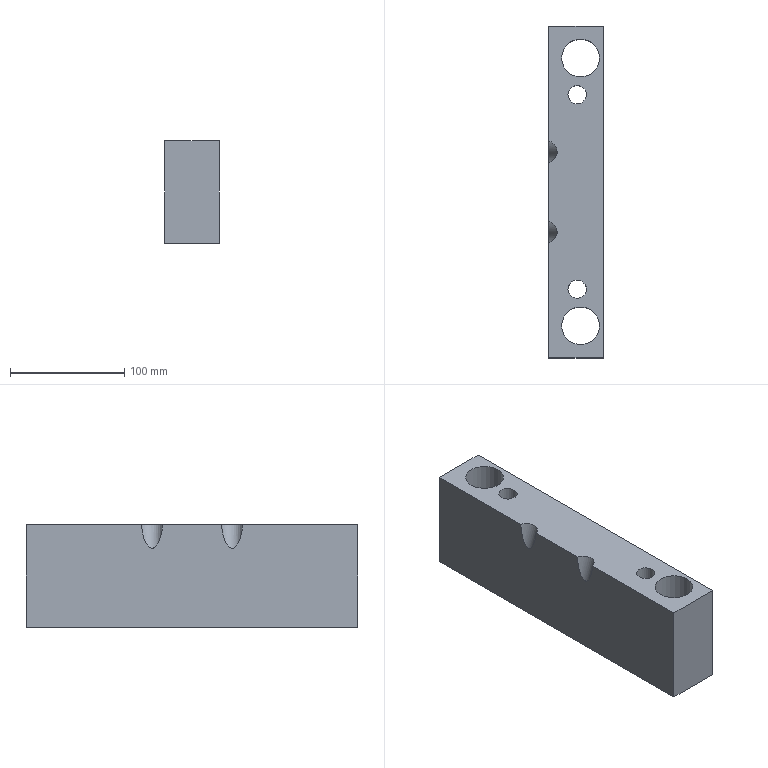Part | STEP file | CC01_id270_x_t | 1 solid | 18 faces | box 48 x 290 x 90 mm | volume 1057434 mm3 | plane 8 | cylinder 8 | cone 2 | commonest cylinder face diameters 10 x2 16 x2 20 x2 33 x2
STEP:
#1=CARTESIAN_POINT('',(-125.,44.563,-75.5));
#2=VERTEX_POINT('',#1);
#3=CARTESIAN_POINT('',(-125.,25.437,-75.5));
#4=VERTEX_POINT('',#3);
#5=CARTESIAN_POINT('',(-125.,35.,-66.95));
#6=DIRECTION('',(-1.,0.,0.));
#7=DIRECTION('',(0.,0.,1.));
#8=AXIS2_PLACEMENT_3D('',#5,#6,#7);
#9=ELLIPSE('',#8,29.238,10.);
#10=EDGE_CURVE('',#2,#4,#9,.T.);
#11=ORIENTED_EDGE('',*,*,#10,.F.);
#12=CARTESIAN_POINT('',(-125.,145.,-75.5));
#13=VERTEX_POINT('',#12);
#14=CARTESIAN_POINT('',(-125.,0.,-75.5));
#15=DIRECTION('',(0.,1.,0.));
#16=VECTOR('',#15,1.);
#17=LINE('',#14,#16);
#18=EDGE_CURVE('',#2,#13,#17,.T.);
#19=ORIENTED_EDGE('',*,*,#18,.T.);
#20=CARTESIAN_POINT('',(-125.,145.,-165.5));
#21=VERTEX_POINT('',#20);
#22=CARTESIAN_POINT('',(-125.,145.,-165.5));
#23=DIRECTION('',(0.,0.,1.));
#24=VECTOR('',#23,1.);
#25=LINE('',#22,#24);
#26=EDGE_CURVE('',#21,#13,#25,.T.);
#27=ORIENTED_EDGE('',*,*,#26,.F.);
#28=CARTESIAN_POINT('',(-125.,-145.,-165.5));
#29=VERTEX_POINT('',#28);
#30=CARTESIAN_POINT('',(-125.,0.,-165.5));
#31=DIRECTION('',(0.,-1.,0.));
#32=VECTOR('',#31,1.);
#33=LINE('',#30,#32);
#34=EDGE_CURVE('',#21,#29,#33,.T.);
#35=ORIENTED_EDGE('',*,*,#34,.T.);
#36=CARTESIAN_POINT('',(-125.,-145.,-75.5));
#37=VERTEX_POINT('',#36);
#38=CARTESIAN_POINT('',(-125.,-145.,-165.5));
#39=DIRECTION('',(0.,0.,1.));
#40=VECTOR('',#39,1.);
#41=LINE('',#38,#40);
#42=EDGE_CURVE('',#29,#37,#41,.T.);
#43=ORIENTED_EDGE('',*,*,#42,.T.);
#44=CARTESIAN_POINT('',(-125.,-44.563,-75.5));
#45=VERTEX_POINT('',#44);
#46=CARTESIAN_POINT('',(-125.,0.,-75.5));
#47=DIRECTION('',(0.,1.,0.));
#48=VECTOR('',#47,1.);
#49=LINE('',#46,#48);
#50=EDGE_CURVE('',#37,#45,#49,.T.);
#51=ORIENTED_EDGE('',*,*,#50,.T.);
#52=CARTESIAN_POINT('',(-125.,-25.437,-75.5));
#53=VERTEX_POINT('',#52);
#54=CARTESIAN_POINT('',(-125.,-35.,-66.95));
#55=DIRECTION('',(-1.,0.,0.));
#56=DIRECTION('',(0.,0.,1.));
#57=AXIS2_PLACEMENT_3D('',#54,#55,#56);
#58=ELLIPSE('',#57,29.238,10.);
#59=EDGE_CURVE('',#53,#45,#58,.T.);
#60=ORIENTED_EDGE('',*,*,#59,.F.);
#61=CARTESIAN_POINT('',(-125.,0.,-75.5));
#62=DIRECTION('',(0.,1.,0.));
#63=VECTOR('',#62,1.);
#64=LINE('',#61,#63);
#65=EDGE_CURVE('',#53,#4,#64,.T.);
#66=ORIENTED_EDGE('',*,*,#65,.T.);
#67=EDGE_LOOP('',(#11,#19,#27,#35,#43,#51,#60,#66));
#68=FACE_OUTER_BOUND('',#67,.T.);
#69=CARTESIAN_POINT('',(-125.,0.,-165.5));
#70=DIRECTION('',(-1.,0.,0.));
#71=DIRECTION('',(0.,0.,1.));
#72=AXIS2_PLACEMENT_3D('',#69,#70,#71);
#73=PLANE('',#72);
#74=ADVANCED_FACE('',(#68),#73,.T.);
#75=CARTESIAN_POINT('',(-113.5,-117.,-165.5));
#76=VERTEX_POINT('',#75);
#77=CARTESIAN_POINT('',(-97.,-117.,-165.5));
#78=DIRECTION('',(0.,0.,1.));
#79=DIRECTION('',(-1.,0.,0.));
#80=AXIS2_PLACEMENT_3D('',#77,#78,#79);
#81=CIRCLE('',#80,16.5);
#82=EDGE_CURVE('',#76,#76,#81,.T.);
#83=ORIENTED_EDGE('',*,*,#82,.T.);
#84=EDGE_LOOP('',(#83));
#85=FACE_BOUND('',#84,.T.);
#86=CARTESIAN_POINT('',(-95.,40.,-165.5));
#87=VERTEX_POINT('',#86);
#88=CARTESIAN_POINT('',(-100.,40.,-165.5));
#89=DIRECTION('',(0.,0.,1.));
#90=DIRECTION('',(1.,0.,0.));
#91=AXIS2_PLACEMENT_3D('',#88,#89,#90);
#92=CIRCLE('',#91,5.);
#93=EDGE_CURVE('',#87,#87,#92,.T.);
#94=ORIENTED_EDGE('',*,*,#93,.T.);
#95=EDGE_LOOP('',(#94));
#96=FACE_BOUND('',#95,.T.);
#97=CARTESIAN_POINT('',(-92.,85.,-165.5));
#98=VERTEX_POINT('',#97);
#99=CARTESIAN_POINT('',(-100.,85.,-165.5));
#100=DIRECTION('',(0.,0.,1.));
#101=DIRECTION('',(1.,0.,0.));
#102=AXIS2_PLACEMENT_3D('',#99,#100,#101);
#103=CIRCLE('',#102,8.);
#104=EDGE_CURVE('',#98,#98,#103,.T.);
#105=ORIENTED_EDGE('',*,*,#104,.T.);
#106=EDGE_LOOP('',(#105));
#107=FACE_BOUND('',#106,.T.);
#108=CARTESIAN_POINT('',(-77.,-145.,-165.5));
#109=VERTEX_POINT('',#108);
#110=CARTESIAN_POINT('',(-77.,145.,-165.5));
#111=VERTEX_POINT('',#110);
#112=CARTESIAN_POINT('',(-77.,0.,-165.5));
#113=DIRECTION('',(0.,1.,0.));
#114=VECTOR('',#113,1.);
#115=LINE('',#112,#114);
#116=EDGE_CURVE('',#109,#111,#115,.T.);
#117=ORIENTED_EDGE('',*,*,#116,.F.);
#118=CARTESIAN_POINT('',(-101.,-145.,-165.5));
#119=DIRECTION('',(1.,0.,0.));
#120=VECTOR('',#119,1.);
#121=LINE('',#118,#120);
#122=EDGE_CURVE('',#29,#109,#121,.T.);
#123=ORIENTED_EDGE('',*,*,#122,.F.);
#124=ORIENTED_EDGE('',*,*,#34,.F.);
#125=CARTESIAN_POINT('',(-101.,145.,-165.5));
#126=DIRECTION('',(-1.,0.,0.));
#127=VECTOR('',#126,1.);
#128=LINE('',#125,#127);
#129=EDGE_CURVE('',#111,#21,#128,.T.);
#130=ORIENTED_EDGE('',*,*,#129,.F.);
#131=EDGE_LOOP('',(#117,#123,#124,#130));
#132=FACE_BOUND('',#131,.T.);
#133=CARTESIAN_POINT('',(-92.,-85.,-165.5));
#134=VERTEX_POINT('',#133);
#135=CARTESIAN_POINT('',(-100.,-85.,-165.5));
#136=DIRECTION('',(0.,0.,1.));
#137=DIRECTION('',(1.,0.,0.));
#138=AXIS2_PLACEMENT_3D('',#135,#136,#137);
#139=CIRCLE('',#138,8.);
#140=EDGE_CURVE('',#134,#134,#139,.T.);
#141=ORIENTED_EDGE('',*,*,#140,.T.);
#142=EDGE_LOOP('',(#141));
#143=FACE_BOUND('',#142,.T.);
#144=CARTESIAN_POINT('',(-95.,-40.,-165.5));
#145=VERTEX_POINT('',#144);
#146=CARTESIAN_POINT('',(-100.,-40.,-165.5));
#147=DIRECTION('',(0.,0.,1.));
#148=DIRECTION('',(1.,0.,0.));
#149=AXIS2_PLACEMENT_3D('',#146,#147,#148);
#150=CIRCLE('',#149,5.);
#151=EDGE_CURVE('',#145,#145,#150,.T.);
#152=ORIENTED_EDGE('',*,*,#151,.T.);
#153=EDGE_LOOP('',(#152));
#154=FACE_BOUND('',#153,.T.);
#155=CARTESIAN_POINT('',(-80.5,117.,-165.5));
#156=VERTEX_POINT('',#155);
#157=CARTESIAN_POINT('',(-97.,117.,-165.5));
#158=DIRECTION('',(0.,0.,1.));
#159=DIRECTION('',(1.,0.,0.));
#160=AXIS2_PLACEMENT_3D('',#157,#158,#159);
#161=CIRCLE('',#160,16.5);
#162=EDGE_CURVE('',#156,#156,#161,.T.);
#163=ORIENTED_EDGE('',*,*,#162,.T.);
#164=EDGE_LOOP('',(#163));
#165=FACE_BOUND('',#164,.T.);
#166=CARTESIAN_POINT('',(-101.,0.,-165.5));
#167=DIRECTION('',(0.,0.,-1.));
#168=DIRECTION('',(-1.,0.,0.));
#169=AXIS2_PLACEMENT_3D('',#166,#167,#168);
#170=PLANE('',#169);
#171=ADVANCED_FACE('',(#85,#96,#107,#132,#143,#154,#165),#170,.T.);
#172=CARTESIAN_POINT('',(-128.112,35.,-75.5));
#173=DIRECTION('',(0.,0.,1.));
#174=DIRECTION('',(1.,0.,0.));
#175=AXIS2_PLACEMENT_3D('',#172,#173,#174);
#176=ELLIPSE('',#175,10.642,10.);
#177=EDGE_CURVE('',#4,#2,#176,.T.);
#178=ORIENTED_EDGE('',*,*,#177,.F.);
#179=ORIENTED_EDGE('',*,*,#65,.F.);
#180=CARTESIAN_POINT('',(-128.112,-35.,-75.5));
#181=DIRECTION('',(0.,0.,1.));
#182=DIRECTION('',(1.,0.,0.));
#183=AXIS2_PLACEMENT_3D('',#180,#181,#182);
#184=ELLIPSE('',#183,10.642,10.);
#185=EDGE_CURVE('',#45,#53,#184,.T.);
#186=ORIENTED_EDGE('',*,*,#185,.F.);
#187=ORIENTED_EDGE('',*,*,#50,.F.);
#188=CARTESIAN_POINT('',(-77.,-145.,-75.5));
#189=VERTEX_POINT('',#188);
#190=CARTESIAN_POINT('',(-101.,-145.,-75.5));
#191=DIRECTION('',(-1.,0.,0.));
#192=VECTOR('',#191,1.);
#193=LINE('',#190,#192);
#194=EDGE_CURVE('',#189,#37,#193,.T.);
#195=ORIENTED_EDGE('',*,*,#194,.F.);
#196=CARTESIAN_POINT('',(-77.,145.,-75.5));
#197=VERTEX_POINT('',#196);
#198=CARTESIAN_POINT('',(-77.,0.,-75.5));
#199=DIRECTION('',(0.,-1.,0.));
#200=VECTOR('',#199,1.);
#201=LINE('',#198,#200);
#202=EDGE_CURVE('',#197,#189,#201,.T.);
#203=ORIENTED_EDGE('',*,*,#202,.F.);
#204=CARTESIAN_POINT('',(-101.,145.,-75.5));
#205=DIRECTION('',(1.,0.,0.));
#206=VECTOR('',#205,1.);
#207=LINE('',#204,#206);
#208=EDGE_CURVE('',#13,#197,#207,.T.);
#209=ORIENTED_EDGE('',*,*,#208,.F.);
#210=ORIENTED_EDGE('',*,*,#18,.F.);
#211=EDGE_LOOP('',(#178,#179,#186,#187,#195,#203,#209,#210));
#212=FACE_BOUND('',#211,.T.);
#213=CARTESIAN_POINT('',(-80.5,-117.,-75.5));
#214=VERTEX_POINT('',#213);
#215=CARTESIAN_POINT('',(-97.,-117.,-75.5));
#216=DIRECTION('',(0.,0.,-1.));
#217=DIRECTION('',(1.,0.,0.));
#218=AXIS2_PLACEMENT_3D('',#215,#216,#217);
#219=CIRCLE('',#218,16.5);
#220=EDGE_CURVE('',#214,#214,#219,.T.);
#221=ORIENTED_EDGE('',*,*,#220,.T.);
#222=EDGE_LOOP('',(#221));
#223=FACE_BOUND('',#222,.T.);
#224=CARTESIAN_POINT('',(-92.,85.,-75.5));
#225=VERTEX_POINT('',#224);
#226=CARTESIAN_POINT('',(-100.,85.,-75.5));
#227=DIRECTION('',(0.,0.,-1.));
#228=DIRECTION('',(1.,0.,0.));
#229=AXIS2_PLACEMENT_3D('',#226,#227,#228);
#230=CIRCLE('',#229,8.);
#231=EDGE_CURVE('',#225,#225,#230,.T.);
#232=ORIENTED_EDGE('',*,*,#231,.T.);
#233=EDGE_LOOP('',(#232));
#234=FACE_BOUND('',#233,.T.);
#235=CARTESIAN_POINT('',(-92.,-85.,-75.5));
#236=VERTEX_POINT('',#235);
#237=CARTESIAN_POINT('',(-100.,-85.,-75.5));
#238=DIRECTION('',(0.,0.,-1.));
#239=DIRECTION('',(1.,0.,0.));
#240=AXIS2_PLACEMENT_3D('',#237,#238,#239);
#241=CIRCLE('',#240,8.);
#242=EDGE_CURVE('',#236,#236,#241,.T.);
#243=ORIENTED_EDGE('',*,*,#242,.T.);
#244=EDGE_LOOP('',(#243));
#245=FACE_BOUND('',#244,.T.);
#246=CARTESIAN_POINT('',(-80.5,117.,-75.5));
#247=VERTEX_POINT('',#246);
#248=CARTESIAN_POINT('',(-97.,117.,-75.5));
#249=DIRECTION('',(0.,0.,-1.));
#250=DIRECTION('',(1.,0.,0.));
#251=AXIS2_PLACEMENT_3D('',#248,#249,#250);
#252=CIRCLE('',#251,16.5);
#253=EDGE_CURVE('',#247,#247,#252,.T.);
#254=ORIENTED_EDGE('',*,*,#253,.T.);
#255=EDGE_LOOP('',(#254));
#256=FACE_BOUND('',#255,.T.);
#257=CARTESIAN_POINT('',(-101.,0.,-75.5));
#258=DIRECTION('',(0.,0.,1.));
#259=DIRECTION('',(1.,0.,0.));
#260=AXIS2_PLACEMENT_3D('',#257,#258,#259);
#261=PLANE('',#260);
#262=ADVANCED_FACE('',(#212,#223,#234,#245,#256),#261,.T.);
#263=CARTESIAN_POINT('',(-77.,-145.,-165.5));
#264=DIRECTION('',(0.,0.,1.));
#265=VECTOR('',#264,1.);
#266=LINE('',#263,#265);
#267=EDGE_CURVE('',#109,#189,#266,.T.);
#268=ORIENTED_EDGE('',*,*,#267,.T.);
#269=ORIENTED_EDGE('',*,*,#194,.T.);
#270=ORIENTED_EDGE('',*,*,#42,.F.);
#271=ORIENTED_EDGE('',*,*,#122,.T.);
#272=EDGE_LOOP('',(#268,#269,#270,#271));
#273=FACE_OUTER_BOUND('',#272,.T.);
#274=CARTESIAN_POINT('',(-101.,-145.,-165.5));
#275=DIRECTION('',(0.,-1.,0.));
#276=DIRECTION('',(0.,0.,-1.));
#277=AXIS2_PLACEMENT_3D('',#274,#275,#276);
#278=PLANE('',#277);
#279=ADVANCED_FACE('',(#273),#278,.T.);
#280=ORIENTED_EDGE('',*,*,#26,.T.);
#281=ORIENTED_EDGE('',*,*,#208,.T.);
#282=CARTESIAN_POINT('',(-77.,145.,-165.5));
#283=DIRECTION('',(0.,0.,1.));
#284=VECTOR('',#283,1.);
#285=LINE('',#282,#284);
#286=EDGE_CURVE('',#111,#197,#285,.T.);
#287=ORIENTED_EDGE('',*,*,#286,.F.);
#288=ORIENTED_EDGE('',*,*,#129,.T.);
#289=EDGE_LOOP('',(#280,#281,#287,#288));
#290=FACE_OUTER_BOUND('',#289,.T.);
#291=CARTESIAN_POINT('',(-101.,145.,-165.5));
#292=DIRECTION('',(0.,1.,0.));
#293=DIRECTION('',(0.,0.,1.));
#294=AXIS2_PLACEMENT_3D('',#291,#292,#293);
#295=PLANE('',#294);
#296=ADVANCED_FACE('',(#290),#295,.T.);
#297=ORIENTED_EDGE('',*,*,#116,.T.);
#298=ORIENTED_EDGE('',*,*,#286,.T.);
#299=ORIENTED_EDGE('',*,*,#202,.T.);
#300=ORIENTED_EDGE('',*,*,#267,.F.);
#301=EDGE_LOOP('',(#297,#298,#299,#300));
#302=FACE_OUTER_BOUND('',#301,.T.);
#303=CARTESIAN_POINT('',(-77.,0.,-165.5));
#304=DIRECTION('',(1.,0.,0.));
#305=DIRECTION('',(0.,0.,-1.));
#306=AXIS2_PLACEMENT_3D('',#303,#304,#305);
#307=PLANE('',#306);
#308=ADVANCED_FACE('',(#302),#307,.T.);
#309=ORIENTED_EDGE('',*,*,#231,.F.);
#310=EDGE_LOOP('',(#309));
#311=FACE_BOUND('',#310,.T.);
#312=ORIENTED_EDGE('',*,*,#104,.F.);
#313=EDGE_LOOP('',(#312));
#314=FACE_BOUND('',#313,.T.);
#315=CARTESIAN_POINT('',(-100.,85.,-165.5));
#316=DIRECTION('',(0.,0.,1.));
#317=DIRECTION('',(1.,0.,0.));
#318=AXIS2_PLACEMENT_3D('',#315,#316,#317);
#319=CYLINDRICAL_SURFACE('',#318,8.);
#320=ADVANCED_FACE('',(#311,#314),#319,.F.);
#321=ORIENTED_EDGE('',*,*,#242,.F.);
#322=EDGE_LOOP('',(#321));
#323=FACE_BOUND('',#322,.T.);
#324=ORIENTED_EDGE('',*,*,#140,.F.);
#325=EDGE_LOOP('',(#324));
#326=FACE_BOUND('',#325,.T.);
#327=CARTESIAN_POINT('',(-100.,-85.,-165.5));
#328=DIRECTION('',(0.,0.,1.));
#329=DIRECTION('',(1.,0.,0.));
#330=AXIS2_PLACEMENT_3D('',#327,#328,#329);
#331=CYLINDRICAL_SURFACE('',#330,8.);
#332=ADVANCED_FACE('',(#323,#326),#331,.F.);
#333=CARTESIAN_POINT('',(-95.5,40.,-144.5));
#334=VERTEX_POINT('',#333);
#335=CARTESIAN_POINT('',(-100.,40.,-144.5));
#336=DIRECTION('',(0.,0.,1.));
#337=DIRECTION('',(1.,0.,0.));
#338=AXIS2_PLACEMENT_3D('',#335,#336,#337);
#339=CIRCLE('',#338,4.5);
#340=EDGE_CURVE('',#334,#334,#339,.T.);
#341=ORIENTED_EDGE('',*,*,#340,.T.);
#342=EDGE_LOOP('',(#341));
#343=FACE_BOUND('',#342,.T.);
#344=CARTESIAN_POINT('',(-105.,40.,-144.5));
#345=VERTEX_POINT('',#344);
#346=CARTESIAN_POINT('',(-100.,40.,-144.5));
#347=DIRECTION('',(0.,0.,-1.));
#348=DIRECTION('',(-1.,0.,0.));
#349=AXIS2_PLACEMENT_3D('',#346,#347,#348);
#350=CIRCLE('',#349,5.);
#351=EDGE_CURVE('',#345,#345,#350,.T.);
#352=ORIENTED_EDGE('',*,*,#351,.T.);
#353=EDGE_LOOP('',(#352));
#354=FACE_BOUND('',#353,.T.);
#355=CARTESIAN_POINT('',(-100.,40.,-144.5));
#356=DIRECTION('',(0.,0.,1.));
#357=DIRECTION('',(1.,0.,0.));
#358=AXIS2_PLACEMENT_3D('',#355,#356,#357);
#359=PLANE('',#358);
#360=ADVANCED_FACE('',(#343,#354),#359,.F.);
#361=ORIENTED_EDGE('',*,*,#351,.F.);
#362=EDGE_LOOP('',(#361));
#363=FACE_BOUND('',#362,.T.);
#364=ORIENTED_EDGE('',*,*,#93,.F.);
#365=EDGE_LOOP('',(#364));
#366=FACE_BOUND('',#365,.T.);
#367=CARTESIAN_POINT('',(-100.,40.,-165.5));
#368=DIRECTION('',(0.,0.,1.));
#369=DIRECTION('',(1.,0.,0.));
#370=AXIS2_PLACEMENT_3D('',#367,#368,#369);
#371=CYLINDRICAL_SURFACE('',#370,5.);
#372=ADVANCED_FACE('',(#363,#366),#371,.F.);
#373=CARTESIAN_POINT('',(-95.5,-40.,-144.5));
#374=VERTEX_POINT('',#373);
#375=CARTESIAN_POINT('',(-100.,-40.,-144.5));
#376=DIRECTION('',(0.,0.,1.));
#377=DIRECTION('',(1.,0.,0.));
#378=AXIS2_PLACEMENT_3D('',#375,#376,#377);
#379=CIRCLE('',#378,4.5);
#380=EDGE_CURVE('',#374,#374,#379,.T.);
#381=ORIENTED_EDGE('',*,*,#380,.T.);
#382=EDGE_LOOP('',(#381));
#383=FACE_BOUND('',#382,.T.);
#384=CARTESIAN_POINT('',(-105.,-40.,-144.5));
#385=VERTEX_POINT('',#384);
#386=CARTESIAN_POINT('',(-100.,-40.,-144.5));
#387=DIRECTION('',(0.,0.,-1.));
#388=DIRECTION('',(-1.,0.,0.));
#389=AXIS2_PLACEMENT_3D('',#386,#387,#388);
#390=CIRCLE('',#389,5.);
#391=EDGE_CURVE('',#385,#385,#390,.T.);
#392=ORIENTED_EDGE('',*,*,#391,.T.);
#393=EDGE_LOOP('',(#392));
#394=FACE_BOUND('',#393,.T.);
#395=CARTESIAN_POINT('',(-100.,-40.,-144.5));
#396=DIRECTION('',(0.,0.,1.));
#397=DIRECTION('',(1.,0.,0.));
#398=AXIS2_PLACEMENT_3D('',#395,#396,#397);
#399=PLANE('',#398);
#400=ADVANCED_FACE('',(#383,#394),#399,.F.);
#401=ORIENTED_EDGE('',*,*,#391,.F.);
#402=EDGE_LOOP('',(#401));
#403=FACE_BOUND('',#402,.T.);
#404=ORIENTED_EDGE('',*,*,#151,.F.);
#405=EDGE_LOOP('',(#404));
#406=FACE_BOUND('',#405,.T.);
#407=CARTESIAN_POINT('',(-100.,-40.,-165.5));
#408=DIRECTION('',(0.,0.,1.));
#409=DIRECTION('',(1.,0.,0.));
#410=AXIS2_PLACEMENT_3D('',#407,#408,#409);
#411=CYLINDRICAL_SURFACE('',#410,5.);
#412=ADVANCED_FACE('',(#403,#406),#411,.F.);
#413=ORIENTED_EDGE('',*,*,#340,.F.);
#414=EDGE_LOOP('',(#413));
#415=FACE_BOUND('',#414,.T.);
#416=CARTESIAN_POINT('',(-100.,40.,-142.05));
#417=VERTEX_POINT('',#416);
#418=VERTEX_LOOP('',#417);
#419=FACE_BOUND('',#418,.T.);
#420=CARTESIAN_POINT('',(-100.,40.,-142.05));
#421=DIRECTION('',(0.,0.,-1.));
#422=DIRECTION('',(-1.,0.,0.));
#423=AXIS2_PLACEMENT_3D('',#420,#421,#422);
#424=CONICAL_SURFACE('',#423,0.,61.434);
#425=ADVANCED_FACE('',(#415,#419),#424,.F.);
#426=ORIENTED_EDGE('',*,*,#380,.F.);
#427=EDGE_LOOP('',(#426));
#428=FACE_BOUND('',#427,.T.);
#429=CARTESIAN_POINT('',(-100.,-40.,-142.05));
#430=VERTEX_POINT('',#429);
#431=VERTEX_LOOP('',#430);
#432=FACE_BOUND('',#431,.T.);
#433=CARTESIAN_POINT('',(-100.,-40.,-142.05));
#434=DIRECTION('',(0.,0.,-1.));
#435=DIRECTION('',(-1.,0.,0.));
#436=AXIS2_PLACEMENT_3D('',#433,#434,#435);
#437=CONICAL_SURFACE('',#436,0.,61.434);
#438=ADVANCED_FACE('',(#428,#432),#437,.F.);
#439=ORIENTED_EDGE('',*,*,#220,.F.);
#440=EDGE_LOOP('',(#439));
#441=FACE_BOUND('',#440,.T.);
#442=ORIENTED_EDGE('',*,*,#82,.F.);
#443=EDGE_LOOP('',(#442));
#444=FACE_BOUND('',#443,.T.);
#445=CARTESIAN_POINT('',(-97.,-117.,-165.5));
#446=DIRECTION('',(0.,0.,1.));
#447=DIRECTION('',(-1.,0.,0.));
#448=AXIS2_PLACEMENT_3D('',#445,#446,#447);
#449=CYLINDRICAL_SURFACE('',#448,16.5);
#450=ADVANCED_FACE('',(#441,#444),#449,.F.);
#451=ORIENTED_EDGE('',*,*,#253,.F.);
#452=EDGE_LOOP('',(#451));
#453=FACE_BOUND('',#452,.T.);
#454=ORIENTED_EDGE('',*,*,#162,.F.);
#455=EDGE_LOOP('',(#454));
#456=FACE_BOUND('',#455,.T.);
#457=CARTESIAN_POINT('',(-97.,117.,-165.5));
#458=DIRECTION('',(0.,0.,1.));
#459=DIRECTION('',(1.,0.,0.));
#460=AXIS2_PLACEMENT_3D('',#457,#458,#459);
#461=CYLINDRICAL_SURFACE('',#460,16.5);
#462=ADVANCED_FACE('',(#453,#456),#461,.F.);
#463=ORIENTED_EDGE('',*,*,#185,.T.);
#464=ORIENTED_EDGE('',*,*,#59,.T.);
#465=EDGE_LOOP('',(#463,#464));
#466=FACE_OUTER_BOUND('',#465,.T.);
#467=CARTESIAN_POINT('',(-105.,-35.,-12.));
#468=DIRECTION('',(0.342,0.,0.9397));
#469=DIRECTION('',(0.9397,0.,-0.342));
#470=AXIS2_PLACEMENT_3D('',#467,#468,#469);
#471=CYLINDRICAL_SURFACE('',#470,10.);
#472=ADVANCED_FACE('',(#466),#471,.F.);
#473=ORIENTED_EDGE('',*,*,#177,.T.);
#474=ORIENTED_EDGE('',*,*,#10,.T.);
#475=EDGE_LOOP('',(#473,#474));
#476=FACE_OUTER_BOUND('',#475,.T.);
#477=CARTESIAN_POINT('',(-105.,35.,-12.));
#478=DIRECTION('',(0.342,0.,0.9397));
#479=DIRECTION('',(0.9397,0.,-0.342));
#480=AXIS2_PLACEMENT_3D('',#477,#478,#479);
#481=CYLINDRICAL_SURFACE('',#480,10.);
#482=ADVANCED_FACE('',(#476),#481,.F.);
#483=CLOSED_SHELL('',(#74,#171,#262,#279,#296,#308,#320,#332,#360,#372,#400,#412,#425,#438,#450,#462,#472,#482));
#484=MANIFOLD_SOLID_BREP('',#483);
#485=(LENGTH_UNIT()NAMED_UNIT(*)SI_UNIT(.MILLI.,.METRE.));
#486=UNCERTAINTY_MEASURE_WITH_UNIT(LENGTH_MEASURE(0.00002),#485,'','');
#487=(NAMED_UNIT(*)PLANE_ANGLE_UNIT()SI_UNIT($,.RADIAN.));
#488=PLANE_ANGLE_MEASURE_WITH_UNIT(PLANE_ANGLE_MEASURE(0.01745),#487);
#489=DIMENSIONAL_EXPONENTS(0.,0.,0.,0.,0.,0.,0.);
#490=(CONVERSION_BASED_UNIT('DEGREE',#488)NAMED_UNIT(#489)PLANE_ANGLE_UNIT());
#491=(NAMED_UNIT(*)SI_UNIT($,.STERADIAN.)SOLID_ANGLE_UNIT());
#492=(GEOMETRIC_REPRESENTATION_CONTEXT(3)GLOBAL_UNCERTAINTY_ASSIGNED_CONTEXT((#486))GLOBAL_UNIT_ASSIGNED_CONTEXT((#485,#490,#491))REPRESENTATION_CONTEXT('',''));
#493=ADVANCED_BREP_SHAPE_REPRESENTATION('',(#484),#492);